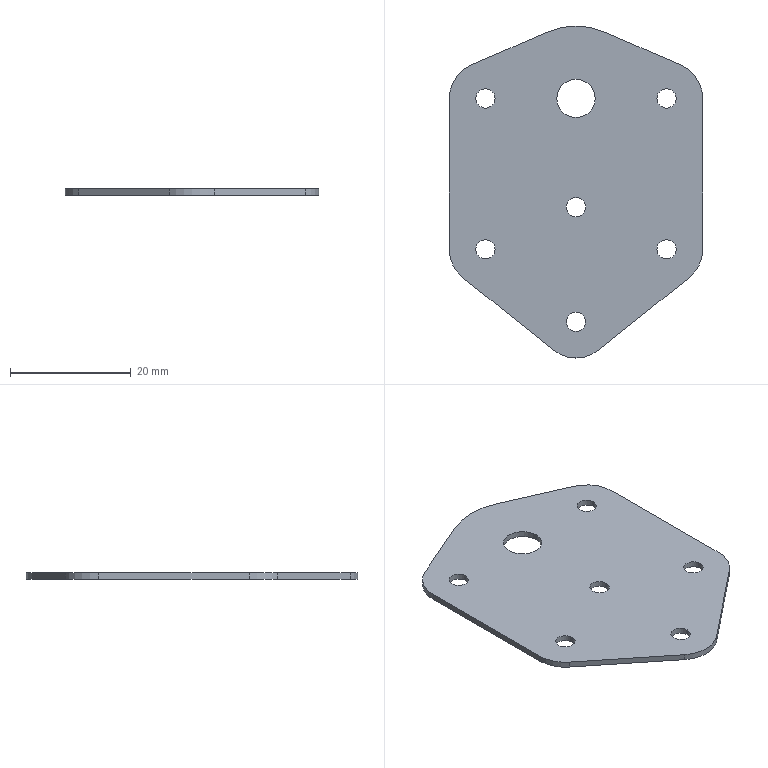Part | SolidWorks | features BaseBody 1 | 1 solid | 28 faces | box 42 x 55 x 1 mm | volume 1786 mm3 | cylinder 20 | plane 8 | commonest cylinder face diameters 3.2 x12 12 x5 6.35 x2 24 x1
STEP:
#1=CARTESIAN_POINT('',(-1.6,-24.5,1.));
#2=VERTEX_POINT('',#1);
#3=CARTESIAN_POINT('',(1.6,-24.5,1.));
#4=VERTEX_POINT('',#3);
#5=CARTESIAN_POINT('',(0.,-24.5,1.));
#6=DIRECTION('',(0.,0.,1.));
#7=DIRECTION('',(-1.,0.,0.));
#8=AXIS2_PLACEMENT_3D('',#5,#6,#7);
#9=CIRCLE('',#8,1.6);
#10=EDGE_CURVE('',#2,#4,#9,.T.);
#11=ORIENTED_EDGE('',*,*,#10,.T.);
#12=CARTESIAN_POINT('',(1.6,-24.5,0.));
#13=VERTEX_POINT('',#12);
#14=CARTESIAN_POINT('',(1.6,-24.5,1.));
#15=DIRECTION('',(0.,0.,-1.));
#16=VECTOR('',#15,1000.);
#17=LINE('',#14,#16);
#18=EDGE_CURVE('',#4,#13,#17,.T.);
#19=ORIENTED_EDGE('',*,*,#18,.T.);
#20=CARTESIAN_POINT('',(-1.6,-24.5,0.));
#21=VERTEX_POINT('',#20);
#22=CARTESIAN_POINT('',(0.,-24.5,0.));
#23=DIRECTION('',(0.,0.,-1.));
#24=DIRECTION('',(-1.,0.,0.));
#25=AXIS2_PLACEMENT_3D('',#22,#23,#24);
#26=CIRCLE('',#25,1.6);
#27=EDGE_CURVE('',#13,#21,#26,.T.);
#28=ORIENTED_EDGE('',*,*,#27,.T.);
#29=CARTESIAN_POINT('',(-1.6,-24.5,1.));
#30=DIRECTION('',(0.,0.,-1.));
#31=VECTOR('',#30,1000.);
#32=LINE('',#29,#31);
#33=EDGE_CURVE('',#2,#21,#32,.T.);
#34=ORIENTED_EDGE('',*,*,#33,.F.);
#35=EDGE_LOOP('',(#11,#19,#28,#34));
#36=FACE_OUTER_BOUND('',#35,.T.);
#37=CARTESIAN_POINT('',(0.,-24.5,1.));
#38=DIRECTION('',(0.,0.,-1.));
#39=DIRECTION('',(-1.,0.,0.));
#40=AXIS2_PLACEMENT_3D('',#37,#38,#39);
#41=CYLINDRICAL_SURFACE('',#40,1.6);
#42=ADVANCED_FACE('',(#36),#41,.F.);
#43=CARTESIAN_POINT('',(1.6,-5.5,1.));
#44=VERTEX_POINT('',#43);
#45=CARTESIAN_POINT('',(-1.6,-5.5,1.));
#46=VERTEX_POINT('',#45);
#47=CARTESIAN_POINT('',(0.,-5.5,1.));
#48=DIRECTION('',(0.,0.,-1.));
#49=DIRECTION('',(-1.,0.,0.));
#50=AXIS2_PLACEMENT_3D('',#47,#48,#49);
#51=CIRCLE('',#50,1.6);
#52=EDGE_CURVE('',#44,#46,#51,.T.);
#53=ORIENTED_EDGE('',*,*,#52,.F.);
#54=CARTESIAN_POINT('',(1.6,-5.5,0.));
#55=VERTEX_POINT('',#54);
#56=CARTESIAN_POINT('',(1.6,-5.5,1.));
#57=DIRECTION('',(0.,0.,-1.));
#58=VECTOR('',#57,1000.);
#59=LINE('',#56,#58);
#60=EDGE_CURVE('',#44,#55,#59,.T.);
#61=ORIENTED_EDGE('',*,*,#60,.T.);
#62=CARTESIAN_POINT('',(-1.6,-5.5,0.));
#63=VERTEX_POINT('',#62);
#64=CARTESIAN_POINT('',(0.,-5.5,0.));
#65=DIRECTION('',(0.,0.,-1.));
#66=DIRECTION('',(-1.,0.,0.));
#67=AXIS2_PLACEMENT_3D('',#64,#65,#66);
#68=CIRCLE('',#67,1.6);
#69=EDGE_CURVE('',#55,#63,#68,.T.);
#70=ORIENTED_EDGE('',*,*,#69,.T.);
#71=CARTESIAN_POINT('',(-1.6,-5.5,1.));
#72=DIRECTION('',(0.,0.,-1.));
#73=VECTOR('',#72,1000.);
#74=LINE('',#71,#73);
#75=EDGE_CURVE('',#46,#63,#74,.T.);
#76=ORIENTED_EDGE('',*,*,#75,.F.);
#77=EDGE_LOOP('',(#53,#61,#70,#76));
#78=FACE_OUTER_BOUND('',#77,.T.);
#79=CARTESIAN_POINT('',(0.,-5.5,1.));
#80=DIRECTION('',(0.,0.,-1.));
#81=DIRECTION('',(-1.,0.,0.));
#82=AXIS2_PLACEMENT_3D('',#79,#80,#81);
#83=CYLINDRICAL_SURFACE('',#82,1.6);
#84=ADVANCED_FACE('',(#78),#83,.F.);
#85=CARTESIAN_POINT('',(-13.4,-12.5,1.));
#86=VERTEX_POINT('',#85);
#87=CARTESIAN_POINT('',(-16.6,-12.5,1.));
#88=VERTEX_POINT('',#87);
#89=CARTESIAN_POINT('',(-15.,-12.5,1.));
#90=DIRECTION('',(0.,0.,-1.));
#91=DIRECTION('',(-1.,0.,0.));
#92=AXIS2_PLACEMENT_3D('',#89,#90,#91);
#93=CIRCLE('',#92,1.6);
#94=EDGE_CURVE('',#86,#88,#93,.T.);
#95=ORIENTED_EDGE('',*,*,#94,.F.);
#96=CARTESIAN_POINT('',(-13.4,-12.5,0.));
#97=VERTEX_POINT('',#96);
#98=CARTESIAN_POINT('',(-13.4,-12.5,1.));
#99=DIRECTION('',(0.,0.,-1.));
#100=VECTOR('',#99,1000.);
#101=LINE('',#98,#100);
#102=EDGE_CURVE('',#86,#97,#101,.T.);
#103=ORIENTED_EDGE('',*,*,#102,.T.);
#104=CARTESIAN_POINT('',(-16.6,-12.5,0.));
#105=VERTEX_POINT('',#104);
#106=CARTESIAN_POINT('',(-15.,-12.5,0.));
#107=DIRECTION('',(0.,0.,-1.));
#108=DIRECTION('',(-1.,0.,0.));
#109=AXIS2_PLACEMENT_3D('',#106,#107,#108);
#110=CIRCLE('',#109,1.6);
#111=EDGE_CURVE('',#97,#105,#110,.T.);
#112=ORIENTED_EDGE('',*,*,#111,.T.);
#113=CARTESIAN_POINT('',(-16.6,-12.5,1.));
#114=DIRECTION('',(0.,0.,-1.));
#115=VECTOR('',#114,1000.);
#116=LINE('',#113,#115);
#117=EDGE_CURVE('',#88,#105,#116,.T.);
#118=ORIENTED_EDGE('',*,*,#117,.F.);
#119=EDGE_LOOP('',(#95,#103,#112,#118));
#120=FACE_OUTER_BOUND('',#119,.T.);
#121=CARTESIAN_POINT('',(-15.,-12.5,1.));
#122=DIRECTION('',(0.,0.,-1.));
#123=DIRECTION('',(-1.,0.,0.));
#124=AXIS2_PLACEMENT_3D('',#121,#122,#123);
#125=CYLINDRICAL_SURFACE('',#124,1.6);
#126=ADVANCED_FACE('',(#120),#125,.F.);
#127=CARTESIAN_POINT('',(-13.4,12.5,1.));
#128=VERTEX_POINT('',#127);
#129=CARTESIAN_POINT('',(-16.6,12.5,1.));
#130=VERTEX_POINT('',#129);
#131=CARTESIAN_POINT('',(-15.,12.5,1.));
#132=DIRECTION('',(0.,0.,-1.));
#133=DIRECTION('',(-1.,0.,0.));
#134=AXIS2_PLACEMENT_3D('',#131,#132,#133);
#135=CIRCLE('',#134,1.6);
#136=EDGE_CURVE('',#128,#130,#135,.T.);
#137=ORIENTED_EDGE('',*,*,#136,.F.);
#138=CARTESIAN_POINT('',(-13.4,12.5,0.));
#139=VERTEX_POINT('',#138);
#140=CARTESIAN_POINT('',(-13.4,12.5,1.));
#141=DIRECTION('',(0.,0.,-1.));
#142=VECTOR('',#141,1000.);
#143=LINE('',#140,#142);
#144=EDGE_CURVE('',#128,#139,#143,.T.);
#145=ORIENTED_EDGE('',*,*,#144,.T.);
#146=CARTESIAN_POINT('',(-16.6,12.5,0.));
#147=VERTEX_POINT('',#146);
#148=CARTESIAN_POINT('',(-15.,12.5,0.));
#149=DIRECTION('',(0.,0.,-1.));
#150=DIRECTION('',(-1.,0.,0.));
#151=AXIS2_PLACEMENT_3D('',#148,#149,#150);
#152=CIRCLE('',#151,1.6);
#153=EDGE_CURVE('',#139,#147,#152,.T.);
#154=ORIENTED_EDGE('',*,*,#153,.T.);
#155=CARTESIAN_POINT('',(-16.6,12.5,1.));
#156=DIRECTION('',(0.,0.,-1.));
#157=VECTOR('',#156,1000.);
#158=LINE('',#155,#157);
#159=EDGE_CURVE('',#130,#147,#158,.T.);
#160=ORIENTED_EDGE('',*,*,#159,.F.);
#161=EDGE_LOOP('',(#137,#145,#154,#160));
#162=FACE_OUTER_BOUND('',#161,.T.);
#163=CARTESIAN_POINT('',(-15.,12.5,1.));
#164=DIRECTION('',(0.,0.,-1.));
#165=DIRECTION('',(-1.,0.,0.));
#166=AXIS2_PLACEMENT_3D('',#163,#164,#165);
#167=CYLINDRICAL_SURFACE('',#166,1.6);
#168=ADVANCED_FACE('',(#162),#167,.F.);
#169=CARTESIAN_POINT('',(16.6,12.5,1.));
#170=VERTEX_POINT('',#169);
#171=CARTESIAN_POINT('',(13.4,12.5,1.));
#172=VERTEX_POINT('',#171);
#173=CARTESIAN_POINT('',(15.,12.5,1.));
#174=DIRECTION('',(0.,0.,-1.));
#175=DIRECTION('',(-1.,0.,0.));
#176=AXIS2_PLACEMENT_3D('',#173,#174,#175);
#177=CIRCLE('',#176,1.6);
#178=EDGE_CURVE('',#170,#172,#177,.T.);
#179=ORIENTED_EDGE('',*,*,#178,.F.);
#180=CARTESIAN_POINT('',(16.6,12.5,0.));
#181=VERTEX_POINT('',#180);
#182=CARTESIAN_POINT('',(16.6,12.5,1.));
#183=DIRECTION('',(0.,0.,-1.));
#184=VECTOR('',#183,1000.);
#185=LINE('',#182,#184);
#186=EDGE_CURVE('',#170,#181,#185,.T.);
#187=ORIENTED_EDGE('',*,*,#186,.T.);
#188=CARTESIAN_POINT('',(13.4,12.5,0.));
#189=VERTEX_POINT('',#188);
#190=CARTESIAN_POINT('',(15.,12.5,0.));
#191=DIRECTION('',(0.,0.,-1.));
#192=DIRECTION('',(-1.,0.,0.));
#193=AXIS2_PLACEMENT_3D('',#190,#191,#192);
#194=CIRCLE('',#193,1.6);
#195=EDGE_CURVE('',#181,#189,#194,.T.);
#196=ORIENTED_EDGE('',*,*,#195,.T.);
#197=CARTESIAN_POINT('',(13.4,12.5,1.));
#198=DIRECTION('',(0.,0.,-1.));
#199=VECTOR('',#198,1000.);
#200=LINE('',#197,#199);
#201=EDGE_CURVE('',#172,#189,#200,.T.);
#202=ORIENTED_EDGE('',*,*,#201,.F.);
#203=EDGE_LOOP('',(#179,#187,#196,#202));
#204=FACE_OUTER_BOUND('',#203,.T.);
#205=CARTESIAN_POINT('',(15.,12.5,1.));
#206=DIRECTION('',(0.,0.,-1.));
#207=DIRECTION('',(-1.,0.,0.));
#208=AXIS2_PLACEMENT_3D('',#205,#206,#207);
#209=CYLINDRICAL_SURFACE('',#208,1.6);
#210=ADVANCED_FACE('',(#204),#209,.F.);
#211=CARTESIAN_POINT('',(16.6,-12.5,1.));
#212=VERTEX_POINT('',#211);
#213=CARTESIAN_POINT('',(13.4,-12.5,1.));
#214=VERTEX_POINT('',#213);
#215=CARTESIAN_POINT('',(15.,-12.5,1.));
#216=DIRECTION('',(0.,0.,-1.));
#217=DIRECTION('',(-1.,0.,0.));
#218=AXIS2_PLACEMENT_3D('',#215,#216,#217);
#219=CIRCLE('',#218,1.6);
#220=EDGE_CURVE('',#212,#214,#219,.T.);
#221=ORIENTED_EDGE('',*,*,#220,.F.);
#222=CARTESIAN_POINT('',(16.6,-12.5,0.));
#223=VERTEX_POINT('',#222);
#224=CARTESIAN_POINT('',(16.6,-12.5,1.));
#225=DIRECTION('',(0.,0.,-1.));
#226=VECTOR('',#225,1000.);
#227=LINE('',#224,#226);
#228=EDGE_CURVE('',#212,#223,#227,.T.);
#229=ORIENTED_EDGE('',*,*,#228,.T.);
#230=CARTESIAN_POINT('',(13.4,-12.5,0.));
#231=VERTEX_POINT('',#230);
#232=CARTESIAN_POINT('',(15.,-12.5,0.));
#233=DIRECTION('',(0.,0.,-1.));
#234=DIRECTION('',(-1.,0.,0.));
#235=AXIS2_PLACEMENT_3D('',#232,#233,#234);
#236=CIRCLE('',#235,1.6);
#237=EDGE_CURVE('',#223,#231,#236,.T.);
#238=ORIENTED_EDGE('',*,*,#237,.T.);
#239=CARTESIAN_POINT('',(13.4,-12.5,1.));
#240=DIRECTION('',(0.,0.,-1.));
#241=VECTOR('',#240,1000.);
#242=LINE('',#239,#241);
#243=EDGE_CURVE('',#214,#231,#242,.T.);
#244=ORIENTED_EDGE('',*,*,#243,.F.);
#245=EDGE_LOOP('',(#221,#229,#238,#244));
#246=FACE_OUTER_BOUND('',#245,.T.);
#247=CARTESIAN_POINT('',(15.,-12.5,1.));
#248=DIRECTION('',(0.,0.,-1.));
#249=DIRECTION('',(-1.,0.,0.));
#250=AXIS2_PLACEMENT_3D('',#247,#248,#249);
#251=CYLINDRICAL_SURFACE('',#250,1.6);
#252=ADVANCED_FACE('',(#246),#251,.F.);
#253=CARTESIAN_POINT('',(3.175,12.5,1.));
#254=VERTEX_POINT('',#253);
#255=CARTESIAN_POINT('',(-3.175,12.5,1.));
#256=VERTEX_POINT('',#255);
#257=CARTESIAN_POINT('',(0.,12.5,1.));
#258=DIRECTION('',(0.,0.,-1.));
#259=DIRECTION('',(-1.,0.,0.));
#260=AXIS2_PLACEMENT_3D('',#257,#258,#259);
#261=CIRCLE('',#260,3.175);
#262=EDGE_CURVE('',#254,#256,#261,.T.);
#263=ORIENTED_EDGE('',*,*,#262,.F.);
#264=CARTESIAN_POINT('',(3.175,12.5,0.));
#265=VERTEX_POINT('',#264);
#266=CARTESIAN_POINT('',(3.175,12.5,1.));
#267=DIRECTION('',(0.,0.,-1.));
#268=VECTOR('',#267,1000.);
#269=LINE('',#266,#268);
#270=EDGE_CURVE('',#254,#265,#269,.T.);
#271=ORIENTED_EDGE('',*,*,#270,.T.);
#272=CARTESIAN_POINT('',(-3.175,12.5,0.));
#273=VERTEX_POINT('',#272);
#274=CARTESIAN_POINT('',(0.,12.5,0.));
#275=DIRECTION('',(0.,0.,-1.));
#276=DIRECTION('',(-1.,0.,0.));
#277=AXIS2_PLACEMENT_3D('',#274,#275,#276);
#278=CIRCLE('',#277,3.175);
#279=EDGE_CURVE('',#265,#273,#278,.T.);
#280=ORIENTED_EDGE('',*,*,#279,.T.);
#281=CARTESIAN_POINT('',(-3.175,12.5,1.));
#282=DIRECTION('',(0.,0.,-1.));
#283=VECTOR('',#282,1000.);
#284=LINE('',#281,#283);
#285=EDGE_CURVE('',#256,#273,#284,.T.);
#286=ORIENTED_EDGE('',*,*,#285,.F.);
#287=EDGE_LOOP('',(#263,#271,#280,#286));
#288=FACE_OUTER_BOUND('',#287,.T.);
#289=CARTESIAN_POINT('',(0.,12.5,1.));
#290=DIRECTION('',(0.,0.,-1.));
#291=DIRECTION('',(-1.,0.,0.));
#292=AXIS2_PLACEMENT_3D('',#289,#290,#291);
#293=CYLINDRICAL_SURFACE('',#292,3.175);
#294=ADVANCED_FACE('',(#288),#293,.F.);
#295=ORIENTED_EDGE('',*,*,#18,.F.);
#296=CARTESIAN_POINT('',(0.,-24.5,1.));
#297=DIRECTION('',(0.,0.,1.));
#298=DIRECTION('',(-1.,0.,0.));
#299=AXIS2_PLACEMENT_3D('',#296,#297,#298);
#300=CIRCLE('',#299,1.6);
#301=EDGE_CURVE('',#4,#2,#300,.T.);
#302=ORIENTED_EDGE('',*,*,#301,.T.);
#303=ORIENTED_EDGE('',*,*,#33,.T.);
#304=CARTESIAN_POINT('',(0.,-24.5,0.));
#305=DIRECTION('',(0.,0.,-1.));
#306=DIRECTION('',(-1.,0.,0.));
#307=AXIS2_PLACEMENT_3D('',#304,#305,#306);
#308=CIRCLE('',#307,1.6);
#309=EDGE_CURVE('',#21,#13,#308,.T.);
#310=ORIENTED_EDGE('',*,*,#309,.T.);
#311=EDGE_LOOP('',(#295,#302,#303,#310));
#312=FACE_OUTER_BOUND('',#311,.T.);
#313=CARTESIAN_POINT('',(0.,-24.5,1.));
#314=DIRECTION('',(0.,0.,-1.));
#315=DIRECTION('',(-1.,0.,0.));
#316=AXIS2_PLACEMENT_3D('',#313,#314,#315);
#317=CYLINDRICAL_SURFACE('',#316,1.6);
#318=ADVANCED_FACE('',(#312),#317,.F.);
#319=ORIENTED_EDGE('',*,*,#309,.F.);
#320=ORIENTED_EDGE('',*,*,#27,.F.);
#321=EDGE_LOOP('',(#319,#320));
#322=FACE_BOUND('',#321,.T.);
#323=CARTESIAN_POINT('',(0.,-5.5,0.));
#324=DIRECTION('',(0.,0.,-1.));
#325=DIRECTION('',(-1.,0.,0.));
#326=AXIS2_PLACEMENT_3D('',#323,#324,#325);
#327=CIRCLE('',#326,1.6);
#328=EDGE_CURVE('',#63,#55,#327,.T.);
#329=ORIENTED_EDGE('',*,*,#328,.F.);
#330=ORIENTED_EDGE('',*,*,#69,.F.);
#331=EDGE_LOOP('',(#329,#330));
#332=FACE_BOUND('',#331,.T.);
#333=CARTESIAN_POINT('',(-15.,-12.5,0.));
#334=DIRECTION('',(0.,0.,-1.));
#335=DIRECTION('',(-1.,0.,0.));
#336=AXIS2_PLACEMENT_3D('',#333,#334,#335);
#337=CIRCLE('',#336,1.6);
#338=EDGE_CURVE('',#105,#97,#337,.T.);
#339=ORIENTED_EDGE('',*,*,#338,.F.);
#340=ORIENTED_EDGE('',*,*,#111,.F.);
#341=EDGE_LOOP('',(#339,#340));
#342=FACE_BOUND('',#341,.T.);
#343=CARTESIAN_POINT('',(-15.,12.5,0.));
#344=DIRECTION('',(0.,0.,-1.));
#345=DIRECTION('',(-1.,0.,0.));
#346=AXIS2_PLACEMENT_3D('',#343,#344,#345);
#347=CIRCLE('',#346,1.6);
#348=EDGE_CURVE('',#147,#139,#347,.T.);
#349=ORIENTED_EDGE('',*,*,#348,.F.);
#350=ORIENTED_EDGE('',*,*,#153,.F.);
#351=EDGE_LOOP('',(#349,#350));
#352=FACE_BOUND('',#351,.T.);
#353=CARTESIAN_POINT('',(15.,12.5,0.));
#354=DIRECTION('',(0.,0.,-1.));
#355=DIRECTION('',(-1.,0.,0.));
#356=AXIS2_PLACEMENT_3D('',#353,#354,#355);
#357=CIRCLE('',#356,1.6);
#358=EDGE_CURVE('',#189,#181,#357,.T.);
#359=ORIENTED_EDGE('',*,*,#358,.F.);
#360=ORIENTED_EDGE('',*,*,#195,.F.);
#361=EDGE_LOOP('',(#359,#360));
#362=FACE_BOUND('',#361,.T.);
#363=CARTESIAN_POINT('',(15.,-12.5,0.));
#364=DIRECTION('',(0.,0.,-1.));
#365=DIRECTION('',(-1.,0.,0.));
#366=AXIS2_PLACEMENT_3D('',#363,#364,#365);
#367=CIRCLE('',#366,1.6);
#368=EDGE_CURVE('',#231,#223,#367,.T.);
#369=ORIENTED_EDGE('',*,*,#368,.F.);
#370=ORIENTED_EDGE('',*,*,#237,.F.);
#371=EDGE_LOOP('',(#369,#370));
#372=FACE_BOUND('',#371,.T.);
#373=CARTESIAN_POINT('',(0.,12.5,0.));
#374=DIRECTION('',(0.,0.,-1.));
#375=DIRECTION('',(-1.,0.,0.));
#376=AXIS2_PLACEMENT_3D('',#373,#374,#375);
#377=CIRCLE('',#376,3.175);
#378=EDGE_CURVE('',#273,#265,#377,.T.);
#379=ORIENTED_EDGE('',*,*,#378,.F.);
#380=ORIENTED_EDGE('',*,*,#279,.F.);
#381=EDGE_LOOP('',(#379,#380));
#382=FACE_BOUND('',#381,.T.);
#383=CARTESIAN_POINT('',(-21.,12.5,0.));
#384=VERTEX_POINT('',#383);
#385=CARTESIAN_POINT('',(-21.,-12.5,0.));
#386=VERTEX_POINT('',#385);
#387=CARTESIAN_POINT('',(-21.,-3.,0.));
#388=DIRECTION('',(0.,-1.,0.));
#389=VECTOR('',#388,1000.);
#390=LINE('',#387,#389);
#391=EDGE_CURVE('',#384,#386,#390,.T.);
#392=ORIENTED_EDGE('',*,*,#391,.F.);
#393=CARTESIAN_POINT('',(-17.4,17.999,0.));
#394=VERTEX_POINT('',#393);
#395=CARTESIAN_POINT('',(-15.,12.5,0.));
#396=DIRECTION('',(0.,0.,1.));
#397=DIRECTION('',(-1.,0.,0.));
#398=AXIS2_PLACEMENT_3D('',#395,#396,#397);
#399=CIRCLE('',#398,6.);
#400=EDGE_CURVE('',#394,#384,#399,.T.);
#401=ORIENTED_EDGE('',*,*,#400,.F.);
#402=CARTESIAN_POINT('',(-4.8,23.498,0.));
#403=VERTEX_POINT('',#402);
#404=CARTESIAN_POINT('',(-17.4,17.999,0.));
#405=DIRECTION('',(-0.9165,-0.4,0.));
#406=VECTOR('',#405,1000.);
#407=LINE('',#404,#406);
#408=EDGE_CURVE('',#403,#394,#407,.T.);
#409=ORIENTED_EDGE('',*,*,#408,.F.);
#410=CARTESIAN_POINT('',(4.8,23.498,0.));
#411=VERTEX_POINT('',#410);
#412=CARTESIAN_POINT('',(0.,12.5,0.));
#413=DIRECTION('',(0.,0.,1.));
#414=DIRECTION('',(-1.,0.,0.));
#415=AXIS2_PLACEMENT_3D('',#412,#413,#414);
#416=CIRCLE('',#415,12.);
#417=EDGE_CURVE('',#411,#403,#416,.T.);
#418=ORIENTED_EDGE('',*,*,#417,.F.);
#419=CARTESIAN_POINT('',(17.4,17.999,0.));
#420=VERTEX_POINT('',#419);
#421=CARTESIAN_POINT('',(4.8,23.498,0.));
#422=DIRECTION('',(-0.9165,0.4,0.));
#423=VECTOR('',#422,1000.);
#424=LINE('',#421,#423);
#425=EDGE_CURVE('',#420,#411,#424,.T.);
#426=ORIENTED_EDGE('',*,*,#425,.F.);
#427=CARTESIAN_POINT('',(21.,12.5,0.));
#428=VERTEX_POINT('',#427);
#429=CARTESIAN_POINT('',(15.,12.5,0.));
#430=DIRECTION('',(0.,0.,1.));
#431=DIRECTION('',(-1.,0.,0.));
#432=AXIS2_PLACEMENT_3D('',#429,#430,#431);
#433=CIRCLE('',#432,6.);
#434=EDGE_CURVE('',#428,#420,#433,.T.);
#435=ORIENTED_EDGE('',*,*,#434,.F.);
#436=CARTESIAN_POINT('',(21.,-12.5,0.));
#437=VERTEX_POINT('',#436);
#438=CARTESIAN_POINT('',(21.,-3.,0.));
#439=DIRECTION('',(0.,1.,0.));
#440=VECTOR('',#439,1000.);
#441=LINE('',#438,#440);
#442=EDGE_CURVE('',#437,#428,#441,.T.);
#443=ORIENTED_EDGE('',*,*,#442,.F.);
#444=CARTESIAN_POINT('',(18.748,-17.185,0.));
#445=VERTEX_POINT('',#444);
#446=CARTESIAN_POINT('',(15.,-12.5,0.));
#447=DIRECTION('',(0.,0.,1.));
#448=DIRECTION('',(-1.,0.,0.));
#449=AXIS2_PLACEMENT_3D('',#446,#447,#448);
#450=CIRCLE('',#449,6.);
#451=EDGE_CURVE('',#445,#437,#450,.T.);
#452=ORIENTED_EDGE('',*,*,#451,.F.);
#453=CARTESIAN_POINT('',(3.748,-29.185,0.));
#454=VERTEX_POINT('',#453);
#455=CARTESIAN_POINT('',(18.748,-17.185,0.));
#456=DIRECTION('',(0.7809,0.6247,0.));
#457=VECTOR('',#456,1000.);
#458=LINE('',#455,#457);
#459=EDGE_CURVE('',#454,#445,#458,.T.);
#460=ORIENTED_EDGE('',*,*,#459,.F.);
#461=CARTESIAN_POINT('',(-3.748,-29.185,0.));
#462=VERTEX_POINT('',#461);
#463=CARTESIAN_POINT('',(0.,-24.5,0.));
#464=DIRECTION('',(0.,0.,1.));
#465=DIRECTION('',(-1.,0.,0.));
#466=AXIS2_PLACEMENT_3D('',#463,#464,#465);
#467=CIRCLE('',#466,6.);
#468=EDGE_CURVE('',#462,#454,#467,.T.);
#469=ORIENTED_EDGE('',*,*,#468,.F.);
#470=CARTESIAN_POINT('',(-18.748,-17.185,0.));
#471=VERTEX_POINT('',#470);
#472=CARTESIAN_POINT('',(-3.748,-29.185,0.));
#473=DIRECTION('',(0.7809,-0.6247,0.));
#474=VECTOR('',#473,1000.);
#475=LINE('',#472,#474);
#476=EDGE_CURVE('',#471,#462,#475,.T.);
#477=ORIENTED_EDGE('',*,*,#476,.F.);
#478=CARTESIAN_POINT('',(-15.,-12.5,0.));
#479=DIRECTION('',(0.,0.,1.));
#480=DIRECTION('',(-1.,0.,0.));
#481=AXIS2_PLACEMENT_3D('',#478,#479,#480);
#482=CIRCLE('',#481,6.);
#483=EDGE_CURVE('',#386,#471,#482,.T.);
#484=ORIENTED_EDGE('',*,*,#483,.F.);
#485=EDGE_LOOP('',(#392,#401,#409,#418,#426,#435,#443,#452,#460,#469,#477,#484));
#486=FACE_OUTER_BOUND('',#485,.T.);
#487=CARTESIAN_POINT('',(-21.,-30.83,0.));
#488=DIRECTION('',(0.,0.,1.));
#489=DIRECTION('',(1.,0.,0.));
#490=AXIS2_PLACEMENT_3D('',#487,#488,#489);
#491=PLANE('',#490);
#492=ADVANCED_FACE('',(#322,#332,#342,#352,#362,#372,#382,#486),#491,.F.);
#493=ORIENTED_EDGE('',*,*,#10,.F.);
#494=ORIENTED_EDGE('',*,*,#301,.F.);
#495=EDGE_LOOP('',(#493,#494));
#496=FACE_BOUND('',#495,.T.);
#497=CARTESIAN_POINT('',(0.,-5.5,1.));
#498=DIRECTION('',(0.,0.,-1.));
#499=DIRECTION('',(-1.,0.,0.));
#500=AXIS2_PLACEMENT_3D('',#497,#498,#499);
#501=CIRCLE('',#500,1.6);
#502=EDGE_CURVE('',#46,#44,#501,.T.);
#503=ORIENTED_EDGE('',*,*,#502,.T.);
#504=ORIENTED_EDGE('',*,*,#52,.T.);
#505=EDGE_LOOP('',(#503,#504));
#506=FACE_BOUND('',#505,.T.);
#507=CARTESIAN_POINT('',(-15.,-12.5,1.));
#508=DIRECTION('',(0.,0.,-1.));
#509=DIRECTION('',(-1.,0.,0.));
#510=AXIS2_PLACEMENT_3D('',#507,#508,#509);
#511=CIRCLE('',#510,1.6);
#512=EDGE_CURVE('',#88,#86,#511,.T.);
#513=ORIENTED_EDGE('',*,*,#512,.T.);
#514=ORIENTED_EDGE('',*,*,#94,.T.);
#515=EDGE_LOOP('',(#513,#514));
#516=FACE_BOUND('',#515,.T.);
#517=CARTESIAN_POINT('',(-15.,12.5,1.));
#518=DIRECTION('',(0.,0.,-1.));
#519=DIRECTION('',(-1.,0.,0.));
#520=AXIS2_PLACEMENT_3D('',#517,#518,#519);
#521=CIRCLE('',#520,1.6);
#522=EDGE_CURVE('',#130,#128,#521,.T.);
#523=ORIENTED_EDGE('',*,*,#522,.T.);
#524=ORIENTED_EDGE('',*,*,#136,.T.);
#525=EDGE_LOOP('',(#523,#524));
#526=FACE_BOUND('',#525,.T.);
#527=CARTESIAN_POINT('',(15.,12.5,1.));
#528=DIRECTION('',(0.,0.,-1.));
#529=DIRECTION('',(-1.,0.,0.));
#530=AXIS2_PLACEMENT_3D('',#527,#528,#529);
#531=CIRCLE('',#530,1.6);
#532=EDGE_CURVE('',#172,#170,#531,.T.);
#533=ORIENTED_EDGE('',*,*,#532,.T.);
#534=ORIENTED_EDGE('',*,*,#178,.T.);
#535=EDGE_LOOP('',(#533,#534));
#536=FACE_BOUND('',#535,.T.);
#537=CARTESIAN_POINT('',(15.,-12.5,1.));
#538=DIRECTION('',(0.,0.,-1.));
#539=DIRECTION('',(-1.,0.,0.));
#540=AXIS2_PLACEMENT_3D('',#537,#538,#539);
#541=CIRCLE('',#540,1.6);
#542=EDGE_CURVE('',#214,#212,#541,.T.);
#543=ORIENTED_EDGE('',*,*,#542,.T.);
#544=ORIENTED_EDGE('',*,*,#220,.T.);
#545=EDGE_LOOP('',(#543,#544));
#546=FACE_BOUND('',#545,.T.);
#547=CARTESIAN_POINT('',(0.,12.5,1.));
#548=DIRECTION('',(0.,0.,-1.));
#549=DIRECTION('',(-1.,0.,0.));
#550=AXIS2_PLACEMENT_3D('',#547,#548,#549);
#551=CIRCLE('',#550,3.175);
#552=EDGE_CURVE('',#256,#254,#551,.T.);
#553=ORIENTED_EDGE('',*,*,#552,.T.);
#554=ORIENTED_EDGE('',*,*,#262,.T.);
#555=EDGE_LOOP('',(#553,#554));
#556=FACE_BOUND('',#555,.T.);
#557=CARTESIAN_POINT('',(-17.4,17.999,1.));
#558=VERTEX_POINT('',#557);
#559=CARTESIAN_POINT('',(-21.,12.5,1.));
#560=VERTEX_POINT('',#559);
#561=CARTESIAN_POINT('',(-15.,12.5,1.));
#562=DIRECTION('',(0.,0.,1.));
#563=DIRECTION('',(-1.,0.,0.));
#564=AXIS2_PLACEMENT_3D('',#561,#562,#563);
#565=CIRCLE('',#564,6.);
#566=EDGE_CURVE('',#558,#560,#565,.T.);
#567=ORIENTED_EDGE('',*,*,#566,.T.);
#568=CARTESIAN_POINT('',(-21.,-12.5,1.));
#569=VERTEX_POINT('',#568);
#570=CARTESIAN_POINT('',(-21.,-3.,1.));
#571=DIRECTION('',(0.,-1.,0.));
#572=VECTOR('',#571,1000.);
#573=LINE('',#570,#572);
#574=EDGE_CURVE('',#560,#569,#573,.T.);
#575=ORIENTED_EDGE('',*,*,#574,.T.);
#576=CARTESIAN_POINT('',(-18.748,-17.185,1.));
#577=VERTEX_POINT('',#576);
#578=CARTESIAN_POINT('',(-15.,-12.5,1.));
#579=DIRECTION('',(0.,0.,1.));
#580=DIRECTION('',(-1.,0.,0.));
#581=AXIS2_PLACEMENT_3D('',#578,#579,#580);
#582=CIRCLE('',#581,6.);
#583=EDGE_CURVE('',#569,#577,#582,.T.);
#584=ORIENTED_EDGE('',*,*,#583,.T.);
#585=CARTESIAN_POINT('',(-3.748,-29.185,1.));
#586=VERTEX_POINT('',#585);
#587=CARTESIAN_POINT('',(-18.748,-17.185,1.));
#588=DIRECTION('',(0.7809,-0.6247,0.));
#589=VECTOR('',#588,1000.);
#590=LINE('',#587,#589);
#591=EDGE_CURVE('',#577,#586,#590,.T.);
#592=ORIENTED_EDGE('',*,*,#591,.T.);
#593=CARTESIAN_POINT('',(3.748,-29.185,1.));
#594=VERTEX_POINT('',#593);
#595=CARTESIAN_POINT('',(0.,-24.5,1.));
#596=DIRECTION('',(0.,0.,1.));
#597=DIRECTION('',(-1.,0.,0.));
#598=AXIS2_PLACEMENT_3D('',#595,#596,#597);
#599=CIRCLE('',#598,6.);
#600=EDGE_CURVE('',#586,#594,#599,.T.);
#601=ORIENTED_EDGE('',*,*,#600,.T.);
#602=CARTESIAN_POINT('',(18.748,-17.185,1.));
#603=VERTEX_POINT('',#602);
#604=CARTESIAN_POINT('',(3.748,-29.185,1.));
#605=DIRECTION('',(0.7809,0.6247,0.));
#606=VECTOR('',#605,1000.);
#607=LINE('',#604,#606);
#608=EDGE_CURVE('',#594,#603,#607,.T.);
#609=ORIENTED_EDGE('',*,*,#608,.T.);
#610=CARTESIAN_POINT('',(21.,-12.5,1.));
#611=VERTEX_POINT('',#610);
#612=CARTESIAN_POINT('',(15.,-12.5,1.));
#613=DIRECTION('',(0.,0.,1.));
#614=DIRECTION('',(-1.,0.,0.));
#615=AXIS2_PLACEMENT_3D('',#612,#613,#614);
#616=CIRCLE('',#615,6.);
#617=EDGE_CURVE('',#603,#611,#616,.T.);
#618=ORIENTED_EDGE('',*,*,#617,.T.);
#619=CARTESIAN_POINT('',(21.,12.5,1.));
#620=VERTEX_POINT('',#619);
#621=CARTESIAN_POINT('',(21.,-3.,1.));
#622=DIRECTION('',(0.,1.,0.));
#623=VECTOR('',#622,1000.);
#624=LINE('',#621,#623);
#625=EDGE_CURVE('',#611,#620,#624,.T.);
#626=ORIENTED_EDGE('',*,*,#625,.T.);
#627=CARTESIAN_POINT('',(17.4,17.999,1.));
#628=VERTEX_POINT('',#627);
#629=CARTESIAN_POINT('',(15.,12.5,1.));
#630=DIRECTION('',(0.,0.,1.));
#631=DIRECTION('',(-1.,0.,0.));
#632=AXIS2_PLACEMENT_3D('',#629,#630,#631);
#633=CIRCLE('',#632,6.);
#634=EDGE_CURVE('',#620,#628,#633,.T.);
#635=ORIENTED_EDGE('',*,*,#634,.T.);
#636=CARTESIAN_POINT('',(4.8,23.498,1.));
#637=VERTEX_POINT('',#636);
#638=CARTESIAN_POINT('',(17.4,17.999,1.));
#639=DIRECTION('',(-0.9165,0.4,0.));
#640=VECTOR('',#639,1000.);
#641=LINE('',#638,#640);
#642=EDGE_CURVE('',#628,#637,#641,.T.);
#643=ORIENTED_EDGE('',*,*,#642,.T.);
#644=CARTESIAN_POINT('',(-4.8,23.498,1.));
#645=VERTEX_POINT('',#644);
#646=CARTESIAN_POINT('',(0.,12.5,1.));
#647=DIRECTION('',(0.,0.,1.));
#648=DIRECTION('',(-1.,0.,0.));
#649=AXIS2_PLACEMENT_3D('',#646,#647,#648);
#650=CIRCLE('',#649,12.);
#651=EDGE_CURVE('',#637,#645,#650,.T.);
#652=ORIENTED_EDGE('',*,*,#651,.T.);
#653=CARTESIAN_POINT('',(-4.8,23.498,1.));
#654=DIRECTION('',(-0.9165,-0.4,0.));
#655=VECTOR('',#654,1000.);
#656=LINE('',#653,#655);
#657=EDGE_CURVE('',#645,#558,#656,.T.);
#658=ORIENTED_EDGE('',*,*,#657,.T.);
#659=EDGE_LOOP('',(#567,#575,#584,#592,#601,#609,#618,#626,#635,#643,#652,#658));
#660=FACE_OUTER_BOUND('',#659,.T.);
#661=CARTESIAN_POINT('',(-21.,-30.83,1.));
#662=DIRECTION('',(0.,0.,1.));
#663=DIRECTION('',(1.,0.,0.));
#664=AXIS2_PLACEMENT_3D('',#661,#662,#663);
#665=PLANE('',#664);
#666=ADVANCED_FACE('',(#496,#506,#516,#526,#536,#546,#556,#660),#665,.T.);
#667=ORIENTED_EDGE('',*,*,#60,.F.);
#668=ORIENTED_EDGE('',*,*,#502,.F.);
#669=ORIENTED_EDGE('',*,*,#75,.T.);
#670=ORIENTED_EDGE('',*,*,#328,.T.);
#671=EDGE_LOOP('',(#667,#668,#669,#670));
#672=FACE_OUTER_BOUND('',#671,.T.);
#673=CARTESIAN_POINT('',(0.,-5.5,1.));
#674=DIRECTION('',(0.,0.,-1.));
#675=DIRECTION('',(-1.,0.,0.));
#676=AXIS2_PLACEMENT_3D('',#673,#674,#675);
#677=CYLINDRICAL_SURFACE('',#676,1.6);
#678=ADVANCED_FACE('',(#672),#677,.F.);
#679=ORIENTED_EDGE('',*,*,#102,.F.);
#680=ORIENTED_EDGE('',*,*,#512,.F.);
#681=ORIENTED_EDGE('',*,*,#117,.T.);
#682=ORIENTED_EDGE('',*,*,#338,.T.);
#683=EDGE_LOOP('',(#679,#680,#681,#682));
#684=FACE_OUTER_BOUND('',#683,.T.);
#685=CARTESIAN_POINT('',(-15.,-12.5,1.));
#686=DIRECTION('',(0.,0.,-1.));
#687=DIRECTION('',(-1.,0.,0.));
#688=AXIS2_PLACEMENT_3D('',#685,#686,#687);
#689=CYLINDRICAL_SURFACE('',#688,1.6);
#690=ADVANCED_FACE('',(#684),#689,.F.);
#691=ORIENTED_EDGE('',*,*,#144,.F.);
#692=ORIENTED_EDGE('',*,*,#522,.F.);
#693=ORIENTED_EDGE('',*,*,#159,.T.);
#694=ORIENTED_EDGE('',*,*,#348,.T.);
#695=EDGE_LOOP('',(#691,#692,#693,#694));
#696=FACE_OUTER_BOUND('',#695,.T.);
#697=CARTESIAN_POINT('',(-15.,12.5,1.));
#698=DIRECTION('',(0.,0.,-1.));
#699=DIRECTION('',(-1.,0.,0.));
#700=AXIS2_PLACEMENT_3D('',#697,#698,#699);
#701=CYLINDRICAL_SURFACE('',#700,1.6);
#702=ADVANCED_FACE('',(#696),#701,.F.);
#703=ORIENTED_EDGE('',*,*,#186,.F.);
#704=ORIENTED_EDGE('',*,*,#532,.F.);
#705=ORIENTED_EDGE('',*,*,#201,.T.);
#706=ORIENTED_EDGE('',*,*,#358,.T.);
#707=EDGE_LOOP('',(#703,#704,#705,#706));
#708=FACE_OUTER_BOUND('',#707,.T.);
#709=CARTESIAN_POINT('',(15.,12.5,1.));
#710=DIRECTION('',(0.,0.,-1.));
#711=DIRECTION('',(-1.,0.,0.));
#712=AXIS2_PLACEMENT_3D('',#709,#710,#711);
#713=CYLINDRICAL_SURFACE('',#712,1.6);
#714=ADVANCED_FACE('',(#708),#713,.F.);
#715=ORIENTED_EDGE('',*,*,#228,.F.);
#716=ORIENTED_EDGE('',*,*,#542,.F.);
#717=ORIENTED_EDGE('',*,*,#243,.T.);
#718=ORIENTED_EDGE('',*,*,#368,.T.);
#719=EDGE_LOOP('',(#715,#716,#717,#718));
#720=FACE_OUTER_BOUND('',#719,.T.);
#721=CARTESIAN_POINT('',(15.,-12.5,1.));
#722=DIRECTION('',(0.,0.,-1.));
#723=DIRECTION('',(-1.,0.,0.));
#724=AXIS2_PLACEMENT_3D('',#721,#722,#723);
#725=CYLINDRICAL_SURFACE('',#724,1.6);
#726=ADVANCED_FACE('',(#720),#725,.F.);
#727=ORIENTED_EDGE('',*,*,#270,.F.);
#728=ORIENTED_EDGE('',*,*,#552,.F.);
#729=ORIENTED_EDGE('',*,*,#285,.T.);
#730=ORIENTED_EDGE('',*,*,#378,.T.);
#731=EDGE_LOOP('',(#727,#728,#729,#730));
#732=FACE_OUTER_BOUND('',#731,.T.);
#733=CARTESIAN_POINT('',(0.,12.5,1.));
#734=DIRECTION('',(0.,0.,-1.));
#735=DIRECTION('',(-1.,0.,0.));
#736=AXIS2_PLACEMENT_3D('',#733,#734,#735);
#737=CYLINDRICAL_SURFACE('',#736,3.175);
#738=ADVANCED_FACE('',(#732),#737,.F.);
#739=CARTESIAN_POINT('',(-18.748,-17.185,0.5));
#740=DIRECTION('',(0.,0.,-1.));
#741=VECTOR('',#740,1000.);
#742=LINE('',#739,#741);
#743=EDGE_CURVE('',#577,#471,#742,.T.);
#744=ORIENTED_EDGE('',*,*,#743,.F.);
#745=ORIENTED_EDGE('',*,*,#583,.F.);
#746=CARTESIAN_POINT('',(-21.,-12.5,0.5));
#747=DIRECTION('',(0.,0.,1.));
#748=VECTOR('',#747,1000.);
#749=LINE('',#746,#748);
#750=EDGE_CURVE('',#386,#569,#749,.T.);
#751=ORIENTED_EDGE('',*,*,#750,.F.);
#752=ORIENTED_EDGE('',*,*,#483,.T.);
#753=EDGE_LOOP('',(#744,#745,#751,#752));
#754=FACE_OUTER_BOUND('',#753,.T.);
#755=CARTESIAN_POINT('',(-15.,-12.5,1.));
#756=DIRECTION('',(0.,0.,-1.));
#757=DIRECTION('',(-1.,0.,0.));
#758=AXIS2_PLACEMENT_3D('',#755,#756,#757);
#759=CYLINDRICAL_SURFACE('',#758,6.);
#760=ADVANCED_FACE('',(#754),#759,.T.);
#761=ORIENTED_EDGE('',*,*,#750,.T.);
#762=ORIENTED_EDGE('',*,*,#574,.F.);
#763=CARTESIAN_POINT('',(-21.,12.5,0.5));
#764=DIRECTION('',(0.,0.,1.));
#765=VECTOR('',#764,1000.);
#766=LINE('',#763,#765);
#767=EDGE_CURVE('',#384,#560,#766,.T.);
#768=ORIENTED_EDGE('',*,*,#767,.F.);
#769=ORIENTED_EDGE('',*,*,#391,.T.);
#770=EDGE_LOOP('',(#761,#762,#768,#769));
#771=FACE_OUTER_BOUND('',#770,.T.);
#772=CARTESIAN_POINT('',(-21.,-12.5,0.));
#773=DIRECTION('',(1.,0.,0.));
#774=DIRECTION('',(0.,1.,0.));
#775=AXIS2_PLACEMENT_3D('',#772,#773,#774);
#776=PLANE('',#775);
#777=ADVANCED_FACE('',(#771),#776,.F.);
#778=ORIENTED_EDGE('',*,*,#767,.T.);
#779=ORIENTED_EDGE('',*,*,#566,.F.);
#780=CARTESIAN_POINT('',(-17.4,17.999,0.5));
#781=DIRECTION('',(0.,0.,1.));
#782=VECTOR('',#781,1000.);
#783=LINE('',#780,#782);
#784=EDGE_CURVE('',#394,#558,#783,.T.);
#785=ORIENTED_EDGE('',*,*,#784,.F.);
#786=ORIENTED_EDGE('',*,*,#400,.T.);
#787=EDGE_LOOP('',(#778,#779,#785,#786));
#788=FACE_OUTER_BOUND('',#787,.T.);
#789=CARTESIAN_POINT('',(-15.,12.5,1.));
#790=DIRECTION('',(0.,0.,-1.));
#791=DIRECTION('',(-1.,0.,0.));
#792=AXIS2_PLACEMENT_3D('',#789,#790,#791);
#793=CYLINDRICAL_SURFACE('',#792,6.);
#794=ADVANCED_FACE('',(#788),#793,.T.);
#795=ORIENTED_EDGE('',*,*,#784,.T.);
#796=ORIENTED_EDGE('',*,*,#657,.F.);
#797=CARTESIAN_POINT('',(-4.8,23.498,0.5));
#798=DIRECTION('',(0.,0.,1.));
#799=VECTOR('',#798,1000.);
#800=LINE('',#797,#799);
#801=EDGE_CURVE('',#403,#645,#800,.T.);
#802=ORIENTED_EDGE('',*,*,#801,.F.);
#803=ORIENTED_EDGE('',*,*,#408,.T.);
#804=EDGE_LOOP('',(#795,#796,#802,#803));
#805=FACE_OUTER_BOUND('',#804,.T.);
#806=CARTESIAN_POINT('',(-17.4,17.999,0.));
#807=DIRECTION('',(0.4,-0.9165,0.));
#808=DIRECTION('',(0.9165,0.4,0.));
#809=AXIS2_PLACEMENT_3D('',#806,#807,#808);
#810=PLANE('',#809);
#811=ADVANCED_FACE('',(#805),#810,.F.);
#812=ORIENTED_EDGE('',*,*,#801,.T.);
#813=ORIENTED_EDGE('',*,*,#651,.F.);
#814=CARTESIAN_POINT('',(4.8,23.498,0.5));
#815=DIRECTION('',(0.,0.,1.));
#816=VECTOR('',#815,1000.);
#817=LINE('',#814,#816);
#818=EDGE_CURVE('',#411,#637,#817,.T.);
#819=ORIENTED_EDGE('',*,*,#818,.F.);
#820=ORIENTED_EDGE('',*,*,#417,.T.);
#821=EDGE_LOOP('',(#812,#813,#819,#820));
#822=FACE_OUTER_BOUND('',#821,.T.);
#823=CARTESIAN_POINT('',(0.,12.5,1.));
#824=DIRECTION('',(0.,0.,-1.));
#825=DIRECTION('',(-1.,0.,0.));
#826=AXIS2_PLACEMENT_3D('',#823,#824,#825);
#827=CYLINDRICAL_SURFACE('',#826,12.);
#828=ADVANCED_FACE('',(#822),#827,.T.);
#829=ORIENTED_EDGE('',*,*,#818,.T.);
#830=ORIENTED_EDGE('',*,*,#642,.F.);
#831=CARTESIAN_POINT('',(17.4,17.999,0.5));
#832=DIRECTION('',(0.,0.,1.));
#833=VECTOR('',#832,1000.);
#834=LINE('',#831,#833);
#835=EDGE_CURVE('',#420,#628,#834,.T.);
#836=ORIENTED_EDGE('',*,*,#835,.F.);
#837=ORIENTED_EDGE('',*,*,#425,.T.);
#838=EDGE_LOOP('',(#829,#830,#836,#837));
#839=FACE_OUTER_BOUND('',#838,.T.);
#840=CARTESIAN_POINT('',(4.8,23.498,0.));
#841=DIRECTION('',(-0.4,-0.9165,0.));
#842=DIRECTION('',(0.9165,-0.4,0.));
#843=AXIS2_PLACEMENT_3D('',#840,#841,#842);
#844=PLANE('',#843);
#845=ADVANCED_FACE('',(#839),#844,.F.);
#846=ORIENTED_EDGE('',*,*,#835,.T.);
#847=ORIENTED_EDGE('',*,*,#634,.F.);
#848=CARTESIAN_POINT('',(21.,12.5,0.5));
#849=DIRECTION('',(0.,0.,1.));
#850=VECTOR('',#849,1000.);
#851=LINE('',#848,#850);
#852=EDGE_CURVE('',#428,#620,#851,.T.);
#853=ORIENTED_EDGE('',*,*,#852,.F.);
#854=ORIENTED_EDGE('',*,*,#434,.T.);
#855=EDGE_LOOP('',(#846,#847,#853,#854));
#856=FACE_OUTER_BOUND('',#855,.T.);
#857=CARTESIAN_POINT('',(15.,12.5,1.));
#858=DIRECTION('',(0.,0.,-1.));
#859=DIRECTION('',(-1.,0.,0.));
#860=AXIS2_PLACEMENT_3D('',#857,#858,#859);
#861=CYLINDRICAL_SURFACE('',#860,6.);
#862=ADVANCED_FACE('',(#856),#861,.T.);
#863=ORIENTED_EDGE('',*,*,#852,.T.);
#864=ORIENTED_EDGE('',*,*,#625,.F.);
#865=CARTESIAN_POINT('',(21.,-12.5,0.5));
#866=DIRECTION('',(0.,0.,1.));
#867=VECTOR('',#866,1000.);
#868=LINE('',#865,#867);
#869=EDGE_CURVE('',#437,#611,#868,.T.);
#870=ORIENTED_EDGE('',*,*,#869,.F.);
#871=ORIENTED_EDGE('',*,*,#442,.T.);
#872=EDGE_LOOP('',(#863,#864,#870,#871));
#873=FACE_OUTER_BOUND('',#872,.T.);
#874=CARTESIAN_POINT('',(21.,12.5,0.));
#875=DIRECTION('',(-1.,0.,0.));
#876=DIRECTION('',(0.,-1.,0.));
#877=AXIS2_PLACEMENT_3D('',#874,#875,#876);
#878=PLANE('',#877);
#879=ADVANCED_FACE('',(#873),#878,.F.);
#880=ORIENTED_EDGE('',*,*,#869,.T.);
#881=ORIENTED_EDGE('',*,*,#617,.F.);
#882=CARTESIAN_POINT('',(18.748,-17.185,0.5));
#883=DIRECTION('',(0.,0.,1.));
#884=VECTOR('',#883,1000.);
#885=LINE('',#882,#884);
#886=EDGE_CURVE('',#445,#603,#885,.T.);
#887=ORIENTED_EDGE('',*,*,#886,.F.);
#888=ORIENTED_EDGE('',*,*,#451,.T.);
#889=EDGE_LOOP('',(#880,#881,#887,#888));
#890=FACE_OUTER_BOUND('',#889,.T.);
#891=CARTESIAN_POINT('',(15.,-12.5,1.));
#892=DIRECTION('',(0.,0.,-1.));
#893=DIRECTION('',(-1.,0.,0.));
#894=AXIS2_PLACEMENT_3D('',#891,#892,#893);
#895=CYLINDRICAL_SURFACE('',#894,6.);
#896=ADVANCED_FACE('',(#890),#895,.T.);
#897=ORIENTED_EDGE('',*,*,#886,.T.);
#898=ORIENTED_EDGE('',*,*,#608,.F.);
#899=CARTESIAN_POINT('',(3.748,-29.185,0.5));
#900=DIRECTION('',(0.,0.,1.));
#901=VECTOR('',#900,1000.);
#902=LINE('',#899,#901);
#903=EDGE_CURVE('',#454,#594,#902,.T.);
#904=ORIENTED_EDGE('',*,*,#903,.F.);
#905=ORIENTED_EDGE('',*,*,#459,.T.);
#906=EDGE_LOOP('',(#897,#898,#904,#905));
#907=FACE_OUTER_BOUND('',#906,.T.);
#908=CARTESIAN_POINT('',(18.748,-17.185,0.));
#909=DIRECTION('',(-0.6247,0.7809,0.));
#910=DIRECTION('',(-0.7809,-0.6247,0.));
#911=AXIS2_PLACEMENT_3D('',#908,#909,#910);
#912=PLANE('',#911);
#913=ADVANCED_FACE('',(#907),#912,.F.);
#914=ORIENTED_EDGE('',*,*,#903,.T.);
#915=ORIENTED_EDGE('',*,*,#600,.F.);
#916=CARTESIAN_POINT('',(-3.748,-29.185,0.5));
#917=DIRECTION('',(0.,0.,1.));
#918=VECTOR('',#917,1000.);
#919=LINE('',#916,#918);
#920=EDGE_CURVE('',#462,#586,#919,.T.);
#921=ORIENTED_EDGE('',*,*,#920,.F.);
#922=ORIENTED_EDGE('',*,*,#468,.T.);
#923=EDGE_LOOP('',(#914,#915,#921,#922));
#924=FACE_OUTER_BOUND('',#923,.T.);
#925=CARTESIAN_POINT('',(0.,-24.5,1.));
#926=DIRECTION('',(0.,0.,-1.));
#927=DIRECTION('',(-1.,0.,0.));
#928=AXIS2_PLACEMENT_3D('',#925,#926,#927);
#929=CYLINDRICAL_SURFACE('',#928,6.);
#930=ADVANCED_FACE('',(#924),#929,.T.);
#931=ORIENTED_EDGE('',*,*,#920,.T.);
#932=ORIENTED_EDGE('',*,*,#591,.F.);
#933=ORIENTED_EDGE('',*,*,#743,.T.);
#934=ORIENTED_EDGE('',*,*,#476,.T.);
#935=EDGE_LOOP('',(#931,#932,#933,#934));
#936=FACE_OUTER_BOUND('',#935,.T.);
#937=CARTESIAN_POINT('',(-3.748,-29.185,0.));
#938=DIRECTION('',(0.6247,0.7809,0.));
#939=DIRECTION('',(-0.7809,0.6247,0.));
#940=AXIS2_PLACEMENT_3D('',#937,#938,#939);
#941=PLANE('',#940);
#942=ADVANCED_FACE('',(#936),#941,.F.);
#943=CLOSED_SHELL('',(#42,#84,#126,#168,#210,#252,#294,#318,#492,#666,#678,#690,#702,#714,#726,#738,#760,#777,#794,#811,#828,#845,#862,#879,#896,#913,#930,#942));
#944=MANIFOLD_SOLID_BREP('',#943);
#945=CARTESIAN_POINT('',(0.,0.,0.));
#946=DIRECTION('',(0.,0.,1.));
#947=DIRECTION('',(1.,0.,0.));
#948=AXIS2_PLACEMENT_3D('',#945,#946,#947);
#949=(LENGTH_UNIT()NAMED_UNIT(*)SI_UNIT(.MILLI.,.METRE.));
#950=UNCERTAINTY_MEASURE_WITH_UNIT(LENGTH_MEASURE(0.00001),#949,'','');
#951=(NAMED_UNIT(*)PLANE_ANGLE_UNIT()SI_UNIT($,.RADIAN.));
#952=(NAMED_UNIT(*)SI_UNIT($,.STERADIAN.)SOLID_ANGLE_UNIT());
#953=(GEOMETRIC_REPRESENTATION_CONTEXT(3)GLOBAL_UNCERTAINTY_ASSIGNED_CONTEXT((#950))GLOBAL_UNIT_ASSIGNED_CONTEXT((#949,#951,#952))REPRESENTATION_CONTEXT('',''));
#954=ADVANCED_BREP_SHAPE_REPRESENTATION('',(#944,#948),#953);